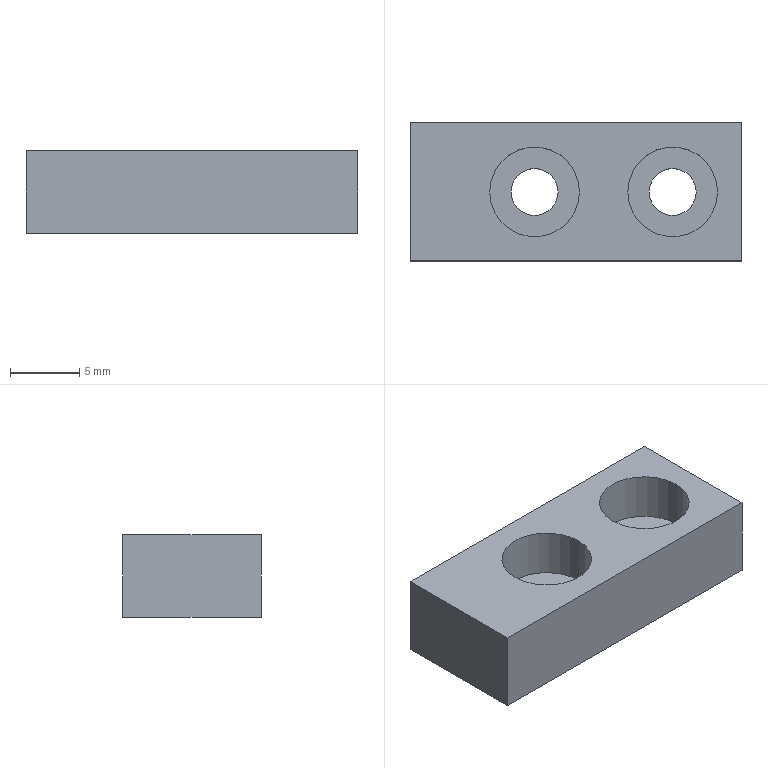Part | STEP file | 0232_211_Slide_Plate | 1 solid | 16 faces | box 24 x 10 x 6 mm | volume 1162 mm3 | cylinder 8 | plane 8 | commonest cylinder face diameters 3.4 x4 6.5 x4
STEP:
#1=CARTESIAN_POINT('',(0.,0.,0.));
#2=DIRECTION('',(0.,0.,1.));
#3=DIRECTION('',(1.,0.,0.));
#4=AXIS2_PLACEMENT_3D('',#1,#2,#3);
#5=CARTESIAN_POINT('',(-11.75,5.,2.5));
#6=VERTEX_POINT('',#5);
#7=CARTESIAN_POINT('',(-11.75,5.,6.));
#8=VERTEX_POINT('',#7);
#9=CARTESIAN_POINT('',(-11.75,5.,6.));
#10=DIRECTION('',(0.,0.,1.));
#11=VECTOR('',#10,1.);
#12=LINE('',#9,#11);
#13=CARTESIAN_POINT('',(-15.,5.,6.));
#14=DIRECTION('',(0.,0.,1.));
#15=DIRECTION('',(1.,0.,0.));
#16=AXIS2_PLACEMENT_3D('',#13,#14,#15);
#17=CYLINDRICAL_SURFACE('',#16,3.25);
#18=CARTESIAN_POINT('',(6.283,0.));
#19=DIRECTION('',(0.,1.));
#20=VECTOR('',#19,1.);
#21=LINE('',#18,#20);
#22=(GEOMETRIC_REPRESENTATION_CONTEXT(2)PARAMETRIC_REPRESENTATION_CONTEXT()REPRESENTATION_CONTEXT('',''));
#23=DEFINITIONAL_REPRESENTATION('',(#21),#22);
#24=PCURVE('',#17,#23);
#25=CARTESIAN_POINT('',(-15.,5.,6.));
#26=DIRECTION('',(0.,0.,1.));
#27=DIRECTION('',(1.,0.,0.));
#28=AXIS2_PLACEMENT_3D('',#25,#26,#27);
#29=CYLINDRICAL_SURFACE('',#28,3.25);
#30=CARTESIAN_POINT('',(0.,0.));
#31=DIRECTION('',(0.,1.));
#32=VECTOR('',#31,1.);
#33=LINE('',#30,#32);
#34=(GEOMETRIC_REPRESENTATION_CONTEXT(2)PARAMETRIC_REPRESENTATION_CONTEXT()REPRESENTATION_CONTEXT('',''));
#35=DEFINITIONAL_REPRESENTATION('',(#33),#34);
#36=PCURVE('',#29,#35);
#37=SURFACE_CURVE('',#12,(#24,#36),.PCURVE_S1.);
#38=EDGE_CURVE('',#6,#8,#37,.T.);
#39=ORIENTED_EDGE('',*,*,#38,.T.);
#40=CARTESIAN_POINT('',(-18.25,5.,6.));
#41=VERTEX_POINT('',#40);
#42=CARTESIAN_POINT('',(-15.,5.,6.));
#43=DIRECTION('',(0.,0.,1.));
#44=DIRECTION('',(1.,0.,0.));
#45=AXIS2_PLACEMENT_3D('',#42,#43,#44);
#46=CIRCLE('',#45,3.25);
#47=CARTESIAN_POINT('',(0.,0.));
#48=DIRECTION('',(1.,0.));
#49=VECTOR('',#48,1.);
#50=LINE('',#47,#49);
#51=(GEOMETRIC_REPRESENTATION_CONTEXT(2)PARAMETRIC_REPRESENTATION_CONTEXT()REPRESENTATION_CONTEXT('',''));
#52=DEFINITIONAL_REPRESENTATION('',(#50),#51);
#53=PCURVE('',#17,#52);
#54=CARTESIAN_POINT('',(-24.,0.,6.));
#55=DIRECTION('',(0.,0.,1.));
#56=DIRECTION('',(1.,0.,0.));
#57=AXIS2_PLACEMENT_3D('',#54,#55,#56);
#58=PLANE('',#57);
#59=CARTESIAN_POINT('',(9.,5.));
#60=DIRECTION('',(1.,0.));
#61=AXIS2_PLACEMENT_2D('',#59,#60);
#62=CIRCLE('',#61,3.25);
#63=(GEOMETRIC_REPRESENTATION_CONTEXT(2)PARAMETRIC_REPRESENTATION_CONTEXT()REPRESENTATION_CONTEXT('',''));
#64=DEFINITIONAL_REPRESENTATION('',(#62),#63);
#65=PCURVE('',#58,#64);
#66=SURFACE_CURVE('',#46,(#53,#65),.PCURVE_S1.);
#67=EDGE_CURVE('',#41,#8,#66,.T.);
#68=ORIENTED_EDGE('',*,*,#67,.F.);
#69=CARTESIAN_POINT('',(-18.25,5.,2.5));
#70=VERTEX_POINT('',#69);
#71=CARTESIAN_POINT('',(-18.25,5.,6.));
#72=DIRECTION('',(0.,0.,1.));
#73=VECTOR('',#72,1.);
#74=LINE('',#71,#73);
#75=CARTESIAN_POINT('',(3.142,0.));
#76=DIRECTION('',(0.,1.));
#77=VECTOR('',#76,1.);
#78=LINE('',#75,#77);
#79=(GEOMETRIC_REPRESENTATION_CONTEXT(2)PARAMETRIC_REPRESENTATION_CONTEXT()REPRESENTATION_CONTEXT('',''));
#80=DEFINITIONAL_REPRESENTATION('',(#78),#79);
#81=PCURVE('',#17,#80);
#82=CARTESIAN_POINT('',(3.142,0.));
#83=DIRECTION('',(0.,1.));
#84=VECTOR('',#83,1.);
#85=LINE('',#82,#84);
#86=(GEOMETRIC_REPRESENTATION_CONTEXT(2)PARAMETRIC_REPRESENTATION_CONTEXT()REPRESENTATION_CONTEXT('',''));
#87=DEFINITIONAL_REPRESENTATION('',(#85),#86);
#88=PCURVE('',#29,#87);
#89=SURFACE_CURVE('',#74,(#81,#88),.PCURVE_S1.);
#90=EDGE_CURVE('',#70,#41,#89,.T.);
#91=ORIENTED_EDGE('',*,*,#90,.F.);
#92=CARTESIAN_POINT('',(-15.,5.,2.5));
#93=DIRECTION('',(0.,0.,1.));
#94=DIRECTION('',(1.,0.,0.));
#95=AXIS2_PLACEMENT_3D('',#92,#93,#94);
#96=CIRCLE('',#95,3.25);
#97=CARTESIAN_POINT('',(0.,-3.5));
#98=DIRECTION('',(1.,0.));
#99=VECTOR('',#98,1.);
#100=LINE('',#97,#99);
#101=(GEOMETRIC_REPRESENTATION_CONTEXT(2)PARAMETRIC_REPRESENTATION_CONTEXT()REPRESENTATION_CONTEXT('',''));
#102=DEFINITIONAL_REPRESENTATION('',(#100),#101);
#103=PCURVE('',#17,#102);
#104=CARTESIAN_POINT('',(-13.3,5.,2.5));
#105=DIRECTION('',(0.,0.,-1.));
#106=DIRECTION('',(-1.,0.,0.));
#107=AXIS2_PLACEMENT_3D('',#104,#105,#106);
#108=PLANE('',#107);
#109=CARTESIAN_POINT('',(-1.55,0.));
#110=CARTESIAN_POINT('',(-1.55,5.629));
#111=CARTESIAN_POINT('',(3.325,2.815));
#112=CARTESIAN_POINT('',(8.2,0.));
#113=CARTESIAN_POINT('',(3.325,-2.815));
#114=CARTESIAN_POINT('',(-1.55,-5.629));
#115=CARTESIAN_POINT('',(-1.55,0.));
#116=(BOUNDED_CURVE()B_SPLINE_CURVE(2,(#109,#110,#111,#112,#113,#114,#115),.UNSPECIFIED.,.T.,.F.)B_SPLINE_CURVE_WITH_KNOTS((1,2,2,2,2,1),(-2.094,0.,2.094,4.189,6.283,8.378),.UNSPECIFIED.)CURVE()GEOMETRIC_REPRESENTATION_ITEM()RATIONAL_B_SPLINE_CURVE((1.,0.5,1.,0.5,1.,0.5,1.))REPRESENTATION_ITEM(''));
#117=(GEOMETRIC_REPRESENTATION_CONTEXT(2)PARAMETRIC_REPRESENTATION_CONTEXT()REPRESENTATION_CONTEXT('',''));
#118=DEFINITIONAL_REPRESENTATION('',(#116),#117);
#119=PCURVE('',#108,#118);
#120=SURFACE_CURVE('',#96,(#103,#119),.PCURVE_S1.);
#121=EDGE_CURVE('',#70,#6,#120,.T.);
#122=ORIENTED_EDGE('',*,*,#121,.T.);
#123=EDGE_LOOP('',(#39,#68,#91,#122));
#124=FACE_BOUND('',#123,.F.);
#125=ADVANCED_FACE('',(#124),#17,.F.);
#126=CARTESIAN_POINT('',(-13.3,5.,0.));
#127=VERTEX_POINT('',#126);
#128=CARTESIAN_POINT('',(-13.3,5.,2.5));
#129=VERTEX_POINT('',#128);
#130=CARTESIAN_POINT('',(-13.3,5.,6.));
#131=DIRECTION('',(0.,0.,1.));
#132=VECTOR('',#131,1.);
#133=LINE('',#130,#132);
#134=CARTESIAN_POINT('',(-15.,5.,6.));
#135=DIRECTION('',(0.,0.,1.));
#136=DIRECTION('',(1.,0.,0.));
#137=AXIS2_PLACEMENT_3D('',#134,#135,#136);
#138=CYLINDRICAL_SURFACE('',#137,1.7);
#139=CARTESIAN_POINT('',(6.283,0.));
#140=DIRECTION('',(0.,1.));
#141=VECTOR('',#140,1.);
#142=LINE('',#139,#141);
#143=(GEOMETRIC_REPRESENTATION_CONTEXT(2)PARAMETRIC_REPRESENTATION_CONTEXT()REPRESENTATION_CONTEXT('',''));
#144=DEFINITIONAL_REPRESENTATION('',(#142),#143);
#145=PCURVE('',#138,#144);
#146=CARTESIAN_POINT('',(-15.,5.,6.));
#147=DIRECTION('',(0.,0.,1.));
#148=DIRECTION('',(1.,0.,0.));
#149=AXIS2_PLACEMENT_3D('',#146,#147,#148);
#150=CYLINDRICAL_SURFACE('',#149,1.7);
#151=CARTESIAN_POINT('',(0.,0.));
#152=DIRECTION('',(0.,1.));
#153=VECTOR('',#152,1.);
#154=LINE('',#151,#153);
#155=(GEOMETRIC_REPRESENTATION_CONTEXT(2)PARAMETRIC_REPRESENTATION_CONTEXT()REPRESENTATION_CONTEXT('',''));
#156=DEFINITIONAL_REPRESENTATION('',(#154),#155);
#157=PCURVE('',#150,#156);
#158=SURFACE_CURVE('',#133,(#145,#157),.PCURVE_S1.);
#159=EDGE_CURVE('',#127,#129,#158,.T.);
#160=ORIENTED_EDGE('',*,*,#159,.T.);
#161=CARTESIAN_POINT('',(-16.7,5.,2.5));
#162=VERTEX_POINT('',#161);
#163=CARTESIAN_POINT('',(-15.,5.,2.5));
#164=DIRECTION('',(0.,0.,1.));
#165=DIRECTION('',(1.,0.,0.));
#166=AXIS2_PLACEMENT_3D('',#163,#164,#165);
#167=CIRCLE('',#166,1.7);
#168=CARTESIAN_POINT('',(0.,-3.5));
#169=DIRECTION('',(1.,0.));
#170=VECTOR('',#169,1.);
#171=LINE('',#168,#170);
#172=(GEOMETRIC_REPRESENTATION_CONTEXT(2)PARAMETRIC_REPRESENTATION_CONTEXT()REPRESENTATION_CONTEXT('',''));
#173=DEFINITIONAL_REPRESENTATION('',(#171),#172);
#174=PCURVE('',#138,#173);
#175=CARTESIAN_POINT('',(0.,0.));
#176=CARTESIAN_POINT('',(0.,2.944));
#177=CARTESIAN_POINT('',(2.55,1.472));
#178=CARTESIAN_POINT('',(5.1,0.));
#179=CARTESIAN_POINT('',(2.55,-1.472));
#180=CARTESIAN_POINT('',(0.,-2.944));
#181=CARTESIAN_POINT('',(0.,0.));
#182=(BOUNDED_CURVE()B_SPLINE_CURVE(2,(#175,#176,#177,#178,#179,#180,#181),.UNSPECIFIED.,.T.,.F.)B_SPLINE_CURVE_WITH_KNOTS((1,2,2,2,2,1),(-2.094,0.,2.094,4.189,6.283,8.378),.UNSPECIFIED.)CURVE()GEOMETRIC_REPRESENTATION_ITEM()RATIONAL_B_SPLINE_CURVE((1.,0.5,1.,0.5,1.,0.5,1.))REPRESENTATION_ITEM(''));
#183=(GEOMETRIC_REPRESENTATION_CONTEXT(2)PARAMETRIC_REPRESENTATION_CONTEXT()REPRESENTATION_CONTEXT('',''));
#184=DEFINITIONAL_REPRESENTATION('',(#182),#183);
#185=PCURVE('',#108,#184);
#186=SURFACE_CURVE('',#167,(#174,#185),.PCURVE_S1.);
#187=EDGE_CURVE('',#162,#129,#186,.T.);
#188=ORIENTED_EDGE('',*,*,#187,.F.);
#189=CARTESIAN_POINT('',(-16.7,5.,0.));
#190=VERTEX_POINT('',#189);
#191=CARTESIAN_POINT('',(-16.7,5.,6.));
#192=DIRECTION('',(0.,0.,1.));
#193=VECTOR('',#192,1.);
#194=LINE('',#191,#193);
#195=CARTESIAN_POINT('',(3.142,0.));
#196=DIRECTION('',(0.,1.));
#197=VECTOR('',#196,1.);
#198=LINE('',#195,#197);
#199=(GEOMETRIC_REPRESENTATION_CONTEXT(2)PARAMETRIC_REPRESENTATION_CONTEXT()REPRESENTATION_CONTEXT('',''));
#200=DEFINITIONAL_REPRESENTATION('',(#198),#199);
#201=PCURVE('',#138,#200);
#202=CARTESIAN_POINT('',(3.142,0.));
#203=DIRECTION('',(0.,1.));
#204=VECTOR('',#203,1.);
#205=LINE('',#202,#204);
#206=(GEOMETRIC_REPRESENTATION_CONTEXT(2)PARAMETRIC_REPRESENTATION_CONTEXT()REPRESENTATION_CONTEXT('',''));
#207=DEFINITIONAL_REPRESENTATION('',(#205),#206);
#208=PCURVE('',#150,#207);
#209=SURFACE_CURVE('',#194,(#201,#208),.PCURVE_S1.);
#210=EDGE_CURVE('',#190,#162,#209,.T.);
#211=ORIENTED_EDGE('',*,*,#210,.F.);
#212=CARTESIAN_POINT('',(-15.,5.,0.));
#213=DIRECTION('',(0.,0.,1.));
#214=DIRECTION('',(1.,0.,0.));
#215=AXIS2_PLACEMENT_3D('',#212,#213,#214);
#216=CIRCLE('',#215,1.7);
#217=CARTESIAN_POINT('',(0.,-6.));
#218=DIRECTION('',(1.,0.));
#219=VECTOR('',#218,1.);
#220=LINE('',#217,#219);
#221=(GEOMETRIC_REPRESENTATION_CONTEXT(2)PARAMETRIC_REPRESENTATION_CONTEXT()REPRESENTATION_CONTEXT('',''));
#222=DEFINITIONAL_REPRESENTATION('',(#220),#221);
#223=PCURVE('',#138,#222);
#224=CARTESIAN_POINT('',(-24.,0.,0.));
#225=DIRECTION('',(0.,0.,1.));
#226=DIRECTION('',(1.,0.,0.));
#227=AXIS2_PLACEMENT_3D('',#224,#225,#226);
#228=PLANE('',#227);
#229=CARTESIAN_POINT('',(9.,5.));
#230=DIRECTION('',(1.,0.));
#231=AXIS2_PLACEMENT_2D('',#229,#230);
#232=CIRCLE('',#231,1.7);
#233=(GEOMETRIC_REPRESENTATION_CONTEXT(2)PARAMETRIC_REPRESENTATION_CONTEXT()REPRESENTATION_CONTEXT('',''));
#234=DEFINITIONAL_REPRESENTATION('',(#232),#233);
#235=PCURVE('',#228,#234);
#236=SURFACE_CURVE('',#216,(#223,#235),.PCURVE_S1.);
#237=EDGE_CURVE('',#190,#127,#236,.T.);
#238=ORIENTED_EDGE('',*,*,#237,.T.);
#239=EDGE_LOOP('',(#160,#188,#211,#238));
#240=FACE_BOUND('',#239,.F.);
#241=ADVANCED_FACE('',(#240),#138,.F.);
#242=CARTESIAN_POINT('',(-1.75,5.,2.5));
#243=VERTEX_POINT('',#242);
#244=CARTESIAN_POINT('',(-1.75,5.,6.));
#245=VERTEX_POINT('',#244);
#246=CARTESIAN_POINT('',(-1.75,5.,6.));
#247=DIRECTION('',(0.,0.,1.));
#248=VECTOR('',#247,1.);
#249=LINE('',#246,#248);
#250=CARTESIAN_POINT('',(-5.,5.,6.));
#251=DIRECTION('',(0.,0.,1.));
#252=DIRECTION('',(1.,0.,0.));
#253=AXIS2_PLACEMENT_3D('',#250,#251,#252);
#254=CYLINDRICAL_SURFACE('',#253,3.25);
#255=CARTESIAN_POINT('',(6.283,0.));
#256=DIRECTION('',(0.,1.));
#257=VECTOR('',#256,1.);
#258=LINE('',#255,#257);
#259=(GEOMETRIC_REPRESENTATION_CONTEXT(2)PARAMETRIC_REPRESENTATION_CONTEXT()REPRESENTATION_CONTEXT('',''));
#260=DEFINITIONAL_REPRESENTATION('',(#258),#259);
#261=PCURVE('',#254,#260);
#262=CARTESIAN_POINT('',(-5.,5.,6.));
#263=DIRECTION('',(0.,0.,1.));
#264=DIRECTION('',(1.,0.,0.));
#265=AXIS2_PLACEMENT_3D('',#262,#263,#264);
#266=CYLINDRICAL_SURFACE('',#265,3.25);
#267=CARTESIAN_POINT('',(0.,0.));
#268=DIRECTION('',(0.,1.));
#269=VECTOR('',#268,1.);
#270=LINE('',#267,#269);
#271=(GEOMETRIC_REPRESENTATION_CONTEXT(2)PARAMETRIC_REPRESENTATION_CONTEXT()REPRESENTATION_CONTEXT('',''));
#272=DEFINITIONAL_REPRESENTATION('',(#270),#271);
#273=PCURVE('',#266,#272);
#274=SURFACE_CURVE('',#249,(#261,#273),.PCURVE_S1.);
#275=EDGE_CURVE('',#243,#245,#274,.T.);
#276=ORIENTED_EDGE('',*,*,#275,.T.);
#277=CARTESIAN_POINT('',(-8.25,5.,6.));
#278=VERTEX_POINT('',#277);
#279=CARTESIAN_POINT('',(-5.,5.,6.));
#280=DIRECTION('',(0.,0.,1.));
#281=DIRECTION('',(1.,0.,0.));
#282=AXIS2_PLACEMENT_3D('',#279,#280,#281);
#283=CIRCLE('',#282,3.25);
#284=CARTESIAN_POINT('',(0.,0.));
#285=DIRECTION('',(1.,0.));
#286=VECTOR('',#285,1.);
#287=LINE('',#284,#286);
#288=(GEOMETRIC_REPRESENTATION_CONTEXT(2)PARAMETRIC_REPRESENTATION_CONTEXT()REPRESENTATION_CONTEXT('',''));
#289=DEFINITIONAL_REPRESENTATION('',(#287),#288);
#290=PCURVE('',#254,#289);
#291=CARTESIAN_POINT('',(19.,5.));
#292=DIRECTION('',(1.,0.));
#293=AXIS2_PLACEMENT_2D('',#291,#292);
#294=CIRCLE('',#293,3.25);
#295=(GEOMETRIC_REPRESENTATION_CONTEXT(2)PARAMETRIC_REPRESENTATION_CONTEXT()REPRESENTATION_CONTEXT('',''));
#296=DEFINITIONAL_REPRESENTATION('',(#294),#295);
#297=PCURVE('',#58,#296);
#298=SURFACE_CURVE('',#283,(#290,#297),.PCURVE_S1.);
#299=EDGE_CURVE('',#278,#245,#298,.T.);
#300=ORIENTED_EDGE('',*,*,#299,.F.);
#301=CARTESIAN_POINT('',(-8.25,5.,2.5));
#302=VERTEX_POINT('',#301);
#303=CARTESIAN_POINT('',(-8.25,5.,6.));
#304=DIRECTION('',(0.,0.,1.));
#305=VECTOR('',#304,1.);
#306=LINE('',#303,#305);
#307=CARTESIAN_POINT('',(3.142,0.));
#308=DIRECTION('',(0.,1.));
#309=VECTOR('',#308,1.);
#310=LINE('',#307,#309);
#311=(GEOMETRIC_REPRESENTATION_CONTEXT(2)PARAMETRIC_REPRESENTATION_CONTEXT()REPRESENTATION_CONTEXT('',''));
#312=DEFINITIONAL_REPRESENTATION('',(#310),#311);
#313=PCURVE('',#254,#312);
#314=CARTESIAN_POINT('',(3.142,0.));
#315=DIRECTION('',(0.,1.));
#316=VECTOR('',#315,1.);
#317=LINE('',#314,#316);
#318=(GEOMETRIC_REPRESENTATION_CONTEXT(2)PARAMETRIC_REPRESENTATION_CONTEXT()REPRESENTATION_CONTEXT('',''));
#319=DEFINITIONAL_REPRESENTATION('',(#317),#318);
#320=PCURVE('',#266,#319);
#321=SURFACE_CURVE('',#306,(#313,#320),.PCURVE_S1.);
#322=EDGE_CURVE('',#302,#278,#321,.T.);
#323=ORIENTED_EDGE('',*,*,#322,.F.);
#324=CARTESIAN_POINT('',(-5.,5.,2.5));
#325=DIRECTION('',(0.,0.,1.));
#326=DIRECTION('',(1.,0.,0.));
#327=AXIS2_PLACEMENT_3D('',#324,#325,#326);
#328=CIRCLE('',#327,3.25);
#329=CARTESIAN_POINT('',(0.,-3.5));
#330=DIRECTION('',(1.,0.));
#331=VECTOR('',#330,1.);
#332=LINE('',#329,#331);
#333=(GEOMETRIC_REPRESENTATION_CONTEXT(2)PARAMETRIC_REPRESENTATION_CONTEXT()REPRESENTATION_CONTEXT('',''));
#334=DEFINITIONAL_REPRESENTATION('',(#332),#333);
#335=PCURVE('',#254,#334);
#336=CARTESIAN_POINT('',(-3.3,5.,2.5));
#337=DIRECTION('',(0.,0.,-1.));
#338=DIRECTION('',(-1.,0.,0.));
#339=AXIS2_PLACEMENT_3D('',#336,#337,#338);
#340=PLANE('',#339);
#341=CARTESIAN_POINT('',(-1.55,0.));
#342=CARTESIAN_POINT('',(-1.55,5.629));
#343=CARTESIAN_POINT('',(3.325,2.815));
#344=CARTESIAN_POINT('',(8.2,0.));
#345=CARTESIAN_POINT('',(3.325,-2.815));
#346=CARTESIAN_POINT('',(-1.55,-5.629));
#347=CARTESIAN_POINT('',(-1.55,0.));
#348=(BOUNDED_CURVE()B_SPLINE_CURVE(2,(#341,#342,#343,#344,#345,#346,#347),.UNSPECIFIED.,.T.,.F.)B_SPLINE_CURVE_WITH_KNOTS((1,2,2,2,2,1),(-2.094,0.,2.094,4.189,6.283,8.378),.UNSPECIFIED.)CURVE()GEOMETRIC_REPRESENTATION_ITEM()RATIONAL_B_SPLINE_CURVE((1.,0.5,1.,0.5,1.,0.5,1.))REPRESENTATION_ITEM(''));
#349=(GEOMETRIC_REPRESENTATION_CONTEXT(2)PARAMETRIC_REPRESENTATION_CONTEXT()REPRESENTATION_CONTEXT('',''));
#350=DEFINITIONAL_REPRESENTATION('',(#348),#349);
#351=PCURVE('',#340,#350);
#352=SURFACE_CURVE('',#328,(#335,#351),.PCURVE_S1.);
#353=EDGE_CURVE('',#302,#243,#352,.T.);
#354=ORIENTED_EDGE('',*,*,#353,.T.);
#355=EDGE_LOOP('',(#276,#300,#323,#354));
#356=FACE_BOUND('',#355,.F.);
#357=ADVANCED_FACE('',(#356),#254,.F.);
#358=CARTESIAN_POINT('',(-3.3,5.,0.));
#359=VERTEX_POINT('',#358);
#360=CARTESIAN_POINT('',(-3.3,5.,2.5));
#361=VERTEX_POINT('',#360);
#362=CARTESIAN_POINT('',(-3.3,5.,6.));
#363=DIRECTION('',(0.,0.,1.));
#364=VECTOR('',#363,1.);
#365=LINE('',#362,#364);
#366=CARTESIAN_POINT('',(-5.,5.,6.));
#367=DIRECTION('',(0.,0.,1.));
#368=DIRECTION('',(1.,0.,0.));
#369=AXIS2_PLACEMENT_3D('',#366,#367,#368);
#370=CYLINDRICAL_SURFACE('',#369,1.7);
#371=CARTESIAN_POINT('',(6.283,0.));
#372=DIRECTION('',(0.,1.));
#373=VECTOR('',#372,1.);
#374=LINE('',#371,#373);
#375=(GEOMETRIC_REPRESENTATION_CONTEXT(2)PARAMETRIC_REPRESENTATION_CONTEXT()REPRESENTATION_CONTEXT('',''));
#376=DEFINITIONAL_REPRESENTATION('',(#374),#375);
#377=PCURVE('',#370,#376);
#378=CARTESIAN_POINT('',(-5.,5.,6.));
#379=DIRECTION('',(0.,0.,1.));
#380=DIRECTION('',(1.,0.,0.));
#381=AXIS2_PLACEMENT_3D('',#378,#379,#380);
#382=CYLINDRICAL_SURFACE('',#381,1.7);
#383=CARTESIAN_POINT('',(0.,0.));
#384=DIRECTION('',(0.,1.));
#385=VECTOR('',#384,1.);
#386=LINE('',#383,#385);
#387=(GEOMETRIC_REPRESENTATION_CONTEXT(2)PARAMETRIC_REPRESENTATION_CONTEXT()REPRESENTATION_CONTEXT('',''));
#388=DEFINITIONAL_REPRESENTATION('',(#386),#387);
#389=PCURVE('',#382,#388);
#390=SURFACE_CURVE('',#365,(#377,#389),.PCURVE_S1.);
#391=EDGE_CURVE('',#359,#361,#390,.T.);
#392=ORIENTED_EDGE('',*,*,#391,.T.);
#393=CARTESIAN_POINT('',(-6.7,5.,2.5));
#394=VERTEX_POINT('',#393);
#395=CARTESIAN_POINT('',(-5.,5.,2.5));
#396=DIRECTION('',(0.,0.,1.));
#397=DIRECTION('',(1.,0.,0.));
#398=AXIS2_PLACEMENT_3D('',#395,#396,#397);
#399=CIRCLE('',#398,1.7);
#400=CARTESIAN_POINT('',(0.,-3.5));
#401=DIRECTION('',(1.,0.));
#402=VECTOR('',#401,1.);
#403=LINE('',#400,#402);
#404=(GEOMETRIC_REPRESENTATION_CONTEXT(2)PARAMETRIC_REPRESENTATION_CONTEXT()REPRESENTATION_CONTEXT('',''));
#405=DEFINITIONAL_REPRESENTATION('',(#403),#404);
#406=PCURVE('',#370,#405);
#407=CARTESIAN_POINT('',(0.,0.));
#408=CARTESIAN_POINT('',(0.,2.944));
#409=CARTESIAN_POINT('',(2.55,1.472));
#410=CARTESIAN_POINT('',(5.1,0.));
#411=CARTESIAN_POINT('',(2.55,-1.472));
#412=CARTESIAN_POINT('',(0.,-2.944));
#413=CARTESIAN_POINT('',(0.,0.));
#414=(BOUNDED_CURVE()B_SPLINE_CURVE(2,(#407,#408,#409,#410,#411,#412,#413),.UNSPECIFIED.,.T.,.F.)B_SPLINE_CURVE_WITH_KNOTS((1,2,2,2,2,1),(-2.094,0.,2.094,4.189,6.283,8.378),.UNSPECIFIED.)CURVE()GEOMETRIC_REPRESENTATION_ITEM()RATIONAL_B_SPLINE_CURVE((1.,0.5,1.,0.5,1.,0.5,1.))REPRESENTATION_ITEM(''));
#415=(GEOMETRIC_REPRESENTATION_CONTEXT(2)PARAMETRIC_REPRESENTATION_CONTEXT()REPRESENTATION_CONTEXT('',''));
#416=DEFINITIONAL_REPRESENTATION('',(#414),#415);
#417=PCURVE('',#340,#416);
#418=SURFACE_CURVE('',#399,(#406,#417),.PCURVE_S1.);
#419=EDGE_CURVE('',#394,#361,#418,.T.);
#420=ORIENTED_EDGE('',*,*,#419,.F.);
#421=CARTESIAN_POINT('',(-6.7,5.,0.));
#422=VERTEX_POINT('',#421);
#423=CARTESIAN_POINT('',(-6.7,5.,6.));
#424=DIRECTION('',(0.,0.,1.));
#425=VECTOR('',#424,1.);
#426=LINE('',#423,#425);
#427=CARTESIAN_POINT('',(3.142,0.));
#428=DIRECTION('',(0.,1.));
#429=VECTOR('',#428,1.);
#430=LINE('',#427,#429);
#431=(GEOMETRIC_REPRESENTATION_CONTEXT(2)PARAMETRIC_REPRESENTATION_CONTEXT()REPRESENTATION_CONTEXT('',''));
#432=DEFINITIONAL_REPRESENTATION('',(#430),#431);
#433=PCURVE('',#370,#432);
#434=CARTESIAN_POINT('',(3.142,0.));
#435=DIRECTION('',(0.,1.));
#436=VECTOR('',#435,1.);
#437=LINE('',#434,#436);
#438=(GEOMETRIC_REPRESENTATION_CONTEXT(2)PARAMETRIC_REPRESENTATION_CONTEXT()REPRESENTATION_CONTEXT('',''));
#439=DEFINITIONAL_REPRESENTATION('',(#437),#438);
#440=PCURVE('',#382,#439);
#441=SURFACE_CURVE('',#426,(#433,#440),.PCURVE_S1.);
#442=EDGE_CURVE('',#422,#394,#441,.T.);
#443=ORIENTED_EDGE('',*,*,#442,.F.);
#444=CARTESIAN_POINT('',(-5.,5.,0.));
#445=DIRECTION('',(0.,0.,1.));
#446=DIRECTION('',(1.,0.,0.));
#447=AXIS2_PLACEMENT_3D('',#444,#445,#446);
#448=CIRCLE('',#447,1.7);
#449=CARTESIAN_POINT('',(0.,-6.));
#450=DIRECTION('',(1.,0.));
#451=VECTOR('',#450,1.);
#452=LINE('',#449,#451);
#453=(GEOMETRIC_REPRESENTATION_CONTEXT(2)PARAMETRIC_REPRESENTATION_CONTEXT()REPRESENTATION_CONTEXT('',''));
#454=DEFINITIONAL_REPRESENTATION('',(#452),#453);
#455=PCURVE('',#370,#454);
#456=CARTESIAN_POINT('',(19.,5.));
#457=DIRECTION('',(1.,0.));
#458=AXIS2_PLACEMENT_2D('',#456,#457);
#459=CIRCLE('',#458,1.7);
#460=(GEOMETRIC_REPRESENTATION_CONTEXT(2)PARAMETRIC_REPRESENTATION_CONTEXT()REPRESENTATION_CONTEXT('',''));
#461=DEFINITIONAL_REPRESENTATION('',(#459),#460);
#462=PCURVE('',#228,#461);
#463=SURFACE_CURVE('',#448,(#455,#462),.PCURVE_S1.);
#464=EDGE_CURVE('',#422,#359,#463,.T.);
#465=ORIENTED_EDGE('',*,*,#464,.T.);
#466=EDGE_LOOP('',(#392,#420,#443,#465));
#467=FACE_BOUND('',#466,.F.);
#468=ADVANCED_FACE('',(#467),#370,.F.);
#469=CARTESIAN_POINT('',(-24.,10.,0.));
#470=VERTEX_POINT('',#469);
#471=CARTESIAN_POINT('',(-24.,0.,0.));
#472=VERTEX_POINT('',#471);
#473=CARTESIAN_POINT('',(-24.,10.,0.));
#474=DIRECTION('',(0.,-1.,0.));
#475=VECTOR('',#474,1.);
#476=LINE('',#473,#475);
#477=CARTESIAN_POINT('',(-24.,10.,6.));
#478=DIRECTION('',(1.,0.,0.));
#479=DIRECTION('',(0.,0.,-1.));
#480=AXIS2_PLACEMENT_3D('',#477,#478,#479);
#481=PLANE('',#480);
#482=CARTESIAN_POINT('',(6.,0.));
#483=DIRECTION('',(0.,-1.));
#484=VECTOR('',#483,1.);
#485=LINE('',#482,#484);
#486=(GEOMETRIC_REPRESENTATION_CONTEXT(2)PARAMETRIC_REPRESENTATION_CONTEXT()REPRESENTATION_CONTEXT('',''));
#487=DEFINITIONAL_REPRESENTATION('',(#485),#486);
#488=PCURVE('',#481,#487);
#489=CARTESIAN_POINT('',(0.,10.));
#490=DIRECTION('',(0.,-1.));
#491=VECTOR('',#490,1.);
#492=LINE('',#489,#491);
#493=(GEOMETRIC_REPRESENTATION_CONTEXT(2)PARAMETRIC_REPRESENTATION_CONTEXT()REPRESENTATION_CONTEXT('',''));
#494=DEFINITIONAL_REPRESENTATION('',(#492),#493);
#495=PCURVE('',#228,#494);
#496=SURFACE_CURVE('',#476,(#488,#495),.PCURVE_S1.);
#497=EDGE_CURVE('',#470,#472,#496,.T.);
#498=ORIENTED_EDGE('',*,*,#497,.T.);
#499=CARTESIAN_POINT('',(-24.,0.,6.));
#500=VERTEX_POINT('',#499);
#501=CARTESIAN_POINT('',(-24.,0.,6.));
#502=DIRECTION('',(0.,0.,-1.));
#503=VECTOR('',#502,1.);
#504=LINE('',#501,#503);
#505=CARTESIAN_POINT('',(0.,-10.));
#506=DIRECTION('',(1.,0.));
#507=VECTOR('',#506,1.);
#508=LINE('',#505,#507);
#509=(GEOMETRIC_REPRESENTATION_CONTEXT(2)PARAMETRIC_REPRESENTATION_CONTEXT()REPRESENTATION_CONTEXT('',''));
#510=DEFINITIONAL_REPRESENTATION('',(#508),#509);
#511=PCURVE('',#481,#510);
#512=CARTESIAN_POINT('',(-24.,0.,6.));
#513=DIRECTION('',(0.,1.,0.));
#514=DIRECTION('',(0.,0.,1.));
#515=AXIS2_PLACEMENT_3D('',#512,#513,#514);
#516=PLANE('',#515);
#517=CARTESIAN_POINT('',(0.,0.));
#518=DIRECTION('',(-1.,0.));
#519=VECTOR('',#518,1.);
#520=LINE('',#517,#519);
#521=(GEOMETRIC_REPRESENTATION_CONTEXT(2)PARAMETRIC_REPRESENTATION_CONTEXT()REPRESENTATION_CONTEXT('',''));
#522=DEFINITIONAL_REPRESENTATION('',(#520),#521);
#523=PCURVE('',#516,#522);
#524=SURFACE_CURVE('',#504,(#511,#523),.PCURVE_S1.);
#525=EDGE_CURVE('',#500,#472,#524,.T.);
#526=ORIENTED_EDGE('',*,*,#525,.F.);
#527=CARTESIAN_POINT('',(-24.,10.,6.));
#528=VERTEX_POINT('',#527);
#529=CARTESIAN_POINT('',(-24.,10.,6.));
#530=DIRECTION('',(0.,-1.,0.));
#531=VECTOR('',#530,1.);
#532=LINE('',#529,#531);
#533=CARTESIAN_POINT('',(0.,0.));
#534=DIRECTION('',(0.,-1.));
#535=VECTOR('',#534,1.);
#536=LINE('',#533,#535);
#537=(GEOMETRIC_REPRESENTATION_CONTEXT(2)PARAMETRIC_REPRESENTATION_CONTEXT()REPRESENTATION_CONTEXT('',''));
#538=DEFINITIONAL_REPRESENTATION('',(#536),#537);
#539=PCURVE('',#481,#538);
#540=CARTESIAN_POINT('',(0.,10.));
#541=DIRECTION('',(0.,-1.));
#542=VECTOR('',#541,1.);
#543=LINE('',#540,#542);
#544=(GEOMETRIC_REPRESENTATION_CONTEXT(2)PARAMETRIC_REPRESENTATION_CONTEXT()REPRESENTATION_CONTEXT('',''));
#545=DEFINITIONAL_REPRESENTATION('',(#543),#544);
#546=PCURVE('',#58,#545);
#547=SURFACE_CURVE('',#532,(#539,#546),.PCURVE_S1.);
#548=EDGE_CURVE('',#528,#500,#547,.T.);
#549=ORIENTED_EDGE('',*,*,#548,.F.);
#550=CARTESIAN_POINT('',(-24.,10.,6.));
#551=DIRECTION('',(0.,0.,-1.));
#552=VECTOR('',#551,1.);
#553=LINE('',#550,#552);
#554=CARTESIAN_POINT('',(0.,0.));
#555=DIRECTION('',(1.,0.));
#556=VECTOR('',#555,1.);
#557=LINE('',#554,#556);
#558=(GEOMETRIC_REPRESENTATION_CONTEXT(2)PARAMETRIC_REPRESENTATION_CONTEXT()REPRESENTATION_CONTEXT('',''));
#559=DEFINITIONAL_REPRESENTATION('',(#557),#558);
#560=PCURVE('',#481,#559);
#561=CARTESIAN_POINT('',(-24.,10.,6.));
#562=DIRECTION('',(0.,-1.,0.));
#563=DIRECTION('',(0.,0.,-1.));
#564=AXIS2_PLACEMENT_3D('',#561,#562,#563);
#565=PLANE('',#564);
#566=CARTESIAN_POINT('',(0.,0.));
#567=DIRECTION('',(1.,0.));
#568=VECTOR('',#567,1.);
#569=LINE('',#566,#568);
#570=(GEOMETRIC_REPRESENTATION_CONTEXT(2)PARAMETRIC_REPRESENTATION_CONTEXT()REPRESENTATION_CONTEXT('',''));
#571=DEFINITIONAL_REPRESENTATION('',(#569),#570);
#572=PCURVE('',#565,#571);
#573=SURFACE_CURVE('',#553,(#560,#572),.PCURVE_S1.);
#574=EDGE_CURVE('',#528,#470,#573,.T.);
#575=ORIENTED_EDGE('',*,*,#574,.T.);
#576=EDGE_LOOP('',(#498,#526,#549,#575));
#577=FACE_BOUND('',#576,.T.);
#578=ADVANCED_FACE('',(#577),#481,.F.);
#579=CARTESIAN_POINT('',(0.,0.,0.));
#580=VERTEX_POINT('',#579);
#581=CARTESIAN_POINT('',(-24.,0.,0.));
#582=DIRECTION('',(1.,0.,0.));
#583=VECTOR('',#582,1.);
#584=LINE('',#581,#583);
#585=CARTESIAN_POINT('',(-6.,0.));
#586=DIRECTION('',(0.,1.));
#587=VECTOR('',#586,1.);
#588=LINE('',#585,#587);
#589=(GEOMETRIC_REPRESENTATION_CONTEXT(2)PARAMETRIC_REPRESENTATION_CONTEXT()REPRESENTATION_CONTEXT('',''));
#590=DEFINITIONAL_REPRESENTATION('',(#588),#589);
#591=PCURVE('',#516,#590);
#592=CARTESIAN_POINT('',(0.,0.));
#593=DIRECTION('',(1.,0.));
#594=VECTOR('',#593,1.);
#595=LINE('',#592,#594);
#596=(GEOMETRIC_REPRESENTATION_CONTEXT(2)PARAMETRIC_REPRESENTATION_CONTEXT()REPRESENTATION_CONTEXT('',''));
#597=DEFINITIONAL_REPRESENTATION('',(#595),#596);
#598=PCURVE('',#228,#597);
#599=SURFACE_CURVE('',#584,(#591,#598),.PCURVE_S1.);
#600=EDGE_CURVE('',#472,#580,#599,.T.);
#601=ORIENTED_EDGE('',*,*,#600,.T.);
#602=CARTESIAN_POINT('',(0.,0.,6.));
#603=VERTEX_POINT('',#602);
#604=CARTESIAN_POINT('',(0.,0.,6.));
#605=DIRECTION('',(0.,0.,-1.));
#606=VECTOR('',#605,1.);
#607=LINE('',#604,#606);
#608=CARTESIAN_POINT('',(0.,24.));
#609=DIRECTION('',(-1.,0.));
#610=VECTOR('',#609,1.);
#611=LINE('',#608,#610);
#612=(GEOMETRIC_REPRESENTATION_CONTEXT(2)PARAMETRIC_REPRESENTATION_CONTEXT()REPRESENTATION_CONTEXT('',''));
#613=DEFINITIONAL_REPRESENTATION('',(#611),#612);
#614=PCURVE('',#516,#613);
#615=CARTESIAN_POINT('',(0.,10.,6.));
#616=DIRECTION('',(-1.,0.,0.));
#617=DIRECTION('',(0.,-1.,0.));
#618=AXIS2_PLACEMENT_3D('',#615,#616,#617);
#619=PLANE('',#618);
#620=CARTESIAN_POINT('',(10.,0.));
#621=DIRECTION('',(0.,-1.));
#622=VECTOR('',#621,1.);
#623=LINE('',#620,#622);
#624=(GEOMETRIC_REPRESENTATION_CONTEXT(2)PARAMETRIC_REPRESENTATION_CONTEXT()REPRESENTATION_CONTEXT('',''));
#625=DEFINITIONAL_REPRESENTATION('',(#623),#624);
#626=PCURVE('',#619,#625);
#627=SURFACE_CURVE('',#607,(#614,#626),.PCURVE_S1.);
#628=EDGE_CURVE('',#603,#580,#627,.T.);
#629=ORIENTED_EDGE('',*,*,#628,.F.);
#630=CARTESIAN_POINT('',(-24.,0.,6.));
#631=DIRECTION('',(1.,0.,0.));
#632=VECTOR('',#631,1.);
#633=LINE('',#630,#632);
#634=CARTESIAN_POINT('',(0.,0.));
#635=DIRECTION('',(0.,1.));
#636=VECTOR('',#635,1.);
#637=LINE('',#634,#636);
#638=(GEOMETRIC_REPRESENTATION_CONTEXT(2)PARAMETRIC_REPRESENTATION_CONTEXT()REPRESENTATION_CONTEXT('',''));
#639=DEFINITIONAL_REPRESENTATION('',(#637),#638);
#640=PCURVE('',#516,#639);
#641=CARTESIAN_POINT('',(0.,0.));
#642=DIRECTION('',(1.,0.));
#643=VECTOR('',#642,1.);
#644=LINE('',#641,#643);
#645=(GEOMETRIC_REPRESENTATION_CONTEXT(2)PARAMETRIC_REPRESENTATION_CONTEXT()REPRESENTATION_CONTEXT('',''));
#646=DEFINITIONAL_REPRESENTATION('',(#644),#645);
#647=PCURVE('',#58,#646);
#648=SURFACE_CURVE('',#633,(#640,#647),.PCURVE_S1.);
#649=EDGE_CURVE('',#500,#603,#648,.T.);
#650=ORIENTED_EDGE('',*,*,#649,.F.);
#651=ORIENTED_EDGE('',*,*,#525,.T.);
#652=EDGE_LOOP('',(#601,#629,#650,#651));
#653=FACE_BOUND('',#652,.T.);
#654=ADVANCED_FACE('',(#653),#516,.F.);
#655=CARTESIAN_POINT('',(0.,10.,0.));
#656=VERTEX_POINT('',#655);
#657=CARTESIAN_POINT('',(0.,10.,0.));
#658=DIRECTION('',(0.,1.,0.));
#659=VECTOR('',#658,1.);
#660=LINE('',#657,#659);
#661=CARTESIAN_POINT('',(0.,-6.));
#662=DIRECTION('',(-1.,0.));
#663=VECTOR('',#662,1.);
#664=LINE('',#661,#663);
#665=(GEOMETRIC_REPRESENTATION_CONTEXT(2)PARAMETRIC_REPRESENTATION_CONTEXT()REPRESENTATION_CONTEXT('',''));
#666=DEFINITIONAL_REPRESENTATION('',(#664),#665);
#667=PCURVE('',#619,#666);
#668=CARTESIAN_POINT('',(24.,10.));
#669=DIRECTION('',(0.,1.));
#670=VECTOR('',#669,1.);
#671=LINE('',#668,#670);
#672=(GEOMETRIC_REPRESENTATION_CONTEXT(2)PARAMETRIC_REPRESENTATION_CONTEXT()REPRESENTATION_CONTEXT('',''));
#673=DEFINITIONAL_REPRESENTATION('',(#671),#672);
#674=PCURVE('',#228,#673);
#675=SURFACE_CURVE('',#660,(#667,#674),.PCURVE_S1.);
#676=EDGE_CURVE('',#580,#656,#675,.T.);
#677=ORIENTED_EDGE('',*,*,#676,.T.);
#678=CARTESIAN_POINT('',(0.,10.,6.));
#679=VERTEX_POINT('',#678);
#680=CARTESIAN_POINT('',(0.,10.,6.));
#681=DIRECTION('',(0.,0.,-1.));
#682=VECTOR('',#681,1.);
#683=LINE('',#680,#682);
#684=CARTESIAN_POINT('',(0.,0.));
#685=DIRECTION('',(0.,-1.));
#686=VECTOR('',#685,1.);
#687=LINE('',#684,#686);
#688=(GEOMETRIC_REPRESENTATION_CONTEXT(2)PARAMETRIC_REPRESENTATION_CONTEXT()REPRESENTATION_CONTEXT('',''));
#689=DEFINITIONAL_REPRESENTATION('',(#687),#688);
#690=PCURVE('',#619,#689);
#691=CARTESIAN_POINT('',(0.,24.));
#692=DIRECTION('',(1.,0.));
#693=VECTOR('',#692,1.);
#694=LINE('',#691,#693);
#695=(GEOMETRIC_REPRESENTATION_CONTEXT(2)PARAMETRIC_REPRESENTATION_CONTEXT()REPRESENTATION_CONTEXT('',''));
#696=DEFINITIONAL_REPRESENTATION('',(#694),#695);
#697=PCURVE('',#565,#696);
#698=SURFACE_CURVE('',#683,(#690,#697),.PCURVE_S1.);
#699=EDGE_CURVE('',#679,#656,#698,.T.);
#700=ORIENTED_EDGE('',*,*,#699,.F.);
#701=CARTESIAN_POINT('',(0.,10.,6.));
#702=DIRECTION('',(0.,1.,0.));
#703=VECTOR('',#702,1.);
#704=LINE('',#701,#703);
#705=CARTESIAN_POINT('',(0.,0.));
#706=DIRECTION('',(-1.,0.));
#707=VECTOR('',#706,1.);
#708=LINE('',#705,#707);
#709=(GEOMETRIC_REPRESENTATION_CONTEXT(2)PARAMETRIC_REPRESENTATION_CONTEXT()REPRESENTATION_CONTEXT('',''));
#710=DEFINITIONAL_REPRESENTATION('',(#708),#709);
#711=PCURVE('',#619,#710);
#712=CARTESIAN_POINT('',(24.,10.));
#713=DIRECTION('',(0.,1.));
#714=VECTOR('',#713,1.);
#715=LINE('',#712,#714);
#716=(GEOMETRIC_REPRESENTATION_CONTEXT(2)PARAMETRIC_REPRESENTATION_CONTEXT()REPRESENTATION_CONTEXT('',''));
#717=DEFINITIONAL_REPRESENTATION('',(#715),#716);
#718=PCURVE('',#58,#717);
#719=SURFACE_CURVE('',#704,(#711,#718),.PCURVE_S1.);
#720=EDGE_CURVE('',#603,#679,#719,.T.);
#721=ORIENTED_EDGE('',*,*,#720,.F.);
#722=ORIENTED_EDGE('',*,*,#628,.T.);
#723=EDGE_LOOP('',(#677,#700,#721,#722));
#724=FACE_BOUND('',#723,.T.);
#725=ADVANCED_FACE('',(#724),#619,.F.);
#726=CARTESIAN_POINT('',(-24.,10.,0.));
#727=DIRECTION('',(-1.,0.,0.));
#728=VECTOR('',#727,1.);
#729=LINE('',#726,#728);
#730=CARTESIAN_POINT('',(6.,0.));
#731=DIRECTION('',(0.,-1.));
#732=VECTOR('',#731,1.);
#733=LINE('',#730,#732);
#734=(GEOMETRIC_REPRESENTATION_CONTEXT(2)PARAMETRIC_REPRESENTATION_CONTEXT()REPRESENTATION_CONTEXT('',''));
#735=DEFINITIONAL_REPRESENTATION('',(#733),#734);
#736=PCURVE('',#565,#735);
#737=CARTESIAN_POINT('',(0.,10.));
#738=DIRECTION('',(-1.,0.));
#739=VECTOR('',#738,1.);
#740=LINE('',#737,#739);
#741=(GEOMETRIC_REPRESENTATION_CONTEXT(2)PARAMETRIC_REPRESENTATION_CONTEXT()REPRESENTATION_CONTEXT('',''));
#742=DEFINITIONAL_REPRESENTATION('',(#740),#741);
#743=PCURVE('',#228,#742);
#744=SURFACE_CURVE('',#729,(#736,#743),.PCURVE_S1.);
#745=EDGE_CURVE('',#656,#470,#744,.T.);
#746=ORIENTED_EDGE('',*,*,#745,.T.);
#747=ORIENTED_EDGE('',*,*,#574,.F.);
#748=CARTESIAN_POINT('',(-24.,10.,6.));
#749=DIRECTION('',(-1.,0.,0.));
#750=VECTOR('',#749,1.);
#751=LINE('',#748,#750);
#752=CARTESIAN_POINT('',(0.,0.));
#753=DIRECTION('',(0.,-1.));
#754=VECTOR('',#753,1.);
#755=LINE('',#752,#754);
#756=(GEOMETRIC_REPRESENTATION_CONTEXT(2)PARAMETRIC_REPRESENTATION_CONTEXT()REPRESENTATION_CONTEXT('',''));
#757=DEFINITIONAL_REPRESENTATION('',(#755),#756);
#758=PCURVE('',#565,#757);
#759=CARTESIAN_POINT('',(0.,10.));
#760=DIRECTION('',(-1.,0.));
#761=VECTOR('',#760,1.);
#762=LINE('',#759,#761);
#763=(GEOMETRIC_REPRESENTATION_CONTEXT(2)PARAMETRIC_REPRESENTATION_CONTEXT()REPRESENTATION_CONTEXT('',''));
#764=DEFINITIONAL_REPRESENTATION('',(#762),#763);
#765=PCURVE('',#58,#764);
#766=SURFACE_CURVE('',#751,(#758,#765),.PCURVE_S1.);
#767=EDGE_CURVE('',#679,#528,#766,.T.);
#768=ORIENTED_EDGE('',*,*,#767,.F.);
#769=ORIENTED_EDGE('',*,*,#699,.T.);
#770=EDGE_LOOP('',(#746,#747,#768,#769));
#771=FACE_BOUND('',#770,.T.);
#772=ADVANCED_FACE('',(#771),#565,.F.);
#773=CARTESIAN_POINT('',(-15.,5.,6.));
#774=DIRECTION('',(0.,0.,1.));
#775=DIRECTION('',(1.,0.,0.));
#776=AXIS2_PLACEMENT_3D('',#773,#774,#775);
#777=CIRCLE('',#776,3.25);
#778=CARTESIAN_POINT('',(9.,5.));
#779=DIRECTION('',(1.,0.));
#780=AXIS2_PLACEMENT_2D('',#778,#779);
#781=CIRCLE('',#780,3.25);
#782=(GEOMETRIC_REPRESENTATION_CONTEXT(2)PARAMETRIC_REPRESENTATION_CONTEXT()REPRESENTATION_CONTEXT('',''));
#783=DEFINITIONAL_REPRESENTATION('',(#781),#782);
#784=PCURVE('',#58,#783);
#785=CARTESIAN_POINT('',(0.,0.));
#786=DIRECTION('',(1.,0.));
#787=VECTOR('',#786,1.);
#788=LINE('',#785,#787);
#789=(GEOMETRIC_REPRESENTATION_CONTEXT(2)PARAMETRIC_REPRESENTATION_CONTEXT()REPRESENTATION_CONTEXT('',''));
#790=DEFINITIONAL_REPRESENTATION('',(#788),#789);
#791=PCURVE('',#29,#790);
#792=SURFACE_CURVE('',#777,(#784,#791),.PCURVE_S1.);
#793=EDGE_CURVE('',#8,#41,#792,.T.);
#794=ORIENTED_EDGE('',*,*,#793,.F.);
#795=ORIENTED_EDGE('',*,*,#67,.F.);
#796=EDGE_LOOP('',(#794,#795));
#797=FACE_BOUND('',#796,.T.);
#798=CARTESIAN_POINT('',(-5.,5.,6.));
#799=DIRECTION('',(0.,0.,1.));
#800=DIRECTION('',(1.,0.,0.));
#801=AXIS2_PLACEMENT_3D('',#798,#799,#800);
#802=CIRCLE('',#801,3.25);
#803=CARTESIAN_POINT('',(19.,5.));
#804=DIRECTION('',(1.,0.));
#805=AXIS2_PLACEMENT_2D('',#803,#804);
#806=CIRCLE('',#805,3.25);
#807=(GEOMETRIC_REPRESENTATION_CONTEXT(2)PARAMETRIC_REPRESENTATION_CONTEXT()REPRESENTATION_CONTEXT('',''));
#808=DEFINITIONAL_REPRESENTATION('',(#806),#807);
#809=PCURVE('',#58,#808);
#810=CARTESIAN_POINT('',(0.,0.));
#811=DIRECTION('',(1.,0.));
#812=VECTOR('',#811,1.);
#813=LINE('',#810,#812);
#814=(GEOMETRIC_REPRESENTATION_CONTEXT(2)PARAMETRIC_REPRESENTATION_CONTEXT()REPRESENTATION_CONTEXT('',''));
#815=DEFINITIONAL_REPRESENTATION('',(#813),#814);
#816=PCURVE('',#266,#815);
#817=SURFACE_CURVE('',#802,(#809,#816),.PCURVE_S1.);
#818=EDGE_CURVE('',#245,#278,#817,.T.);
#819=ORIENTED_EDGE('',*,*,#818,.F.);
#820=ORIENTED_EDGE('',*,*,#299,.F.);
#821=EDGE_LOOP('',(#819,#820));
#822=FACE_BOUND('',#821,.T.);
#823=ORIENTED_EDGE('',*,*,#548,.T.);
#824=ORIENTED_EDGE('',*,*,#649,.T.);
#825=ORIENTED_EDGE('',*,*,#720,.T.);
#826=ORIENTED_EDGE('',*,*,#767,.T.);
#827=EDGE_LOOP('',(#823,#824,#825,#826));
#828=FACE_BOUND('',#827,.T.);
#829=ADVANCED_FACE('',(#797,#822,#828),#58,.T.);
#830=CARTESIAN_POINT('',(-15.,5.,0.));
#831=DIRECTION('',(0.,0.,1.));
#832=DIRECTION('',(1.,0.,0.));
#833=AXIS2_PLACEMENT_3D('',#830,#831,#832);
#834=CIRCLE('',#833,1.7);
#835=CARTESIAN_POINT('',(9.,5.));
#836=DIRECTION('',(1.,0.));
#837=AXIS2_PLACEMENT_2D('',#835,#836);
#838=CIRCLE('',#837,1.7);
#839=(GEOMETRIC_REPRESENTATION_CONTEXT(2)PARAMETRIC_REPRESENTATION_CONTEXT()REPRESENTATION_CONTEXT('',''));
#840=DEFINITIONAL_REPRESENTATION('',(#838),#839);
#841=PCURVE('',#228,#840);
#842=CARTESIAN_POINT('',(0.,-6.));
#843=DIRECTION('',(1.,0.));
#844=VECTOR('',#843,1.);
#845=LINE('',#842,#844);
#846=(GEOMETRIC_REPRESENTATION_CONTEXT(2)PARAMETRIC_REPRESENTATION_CONTEXT()REPRESENTATION_CONTEXT('',''));
#847=DEFINITIONAL_REPRESENTATION('',(#845),#846);
#848=PCURVE('',#150,#847);
#849=SURFACE_CURVE('',#834,(#841,#848),.PCURVE_S1.);
#850=EDGE_CURVE('',#127,#190,#849,.T.);
#851=ORIENTED_EDGE('',*,*,#850,.T.);
#852=ORIENTED_EDGE('',*,*,#237,.T.);
#853=EDGE_LOOP('',(#851,#852));
#854=FACE_BOUND('',#853,.T.);
#855=CARTESIAN_POINT('',(-5.,5.,0.));
#856=DIRECTION('',(0.,0.,1.));
#857=DIRECTION('',(1.,0.,0.));
#858=AXIS2_PLACEMENT_3D('',#855,#856,#857);
#859=CIRCLE('',#858,1.7);
#860=CARTESIAN_POINT('',(19.,5.));
#861=DIRECTION('',(1.,0.));
#862=AXIS2_PLACEMENT_2D('',#860,#861);
#863=CIRCLE('',#862,1.7);
#864=(GEOMETRIC_REPRESENTATION_CONTEXT(2)PARAMETRIC_REPRESENTATION_CONTEXT()REPRESENTATION_CONTEXT('',''));
#865=DEFINITIONAL_REPRESENTATION('',(#863),#864);
#866=PCURVE('',#228,#865);
#867=CARTESIAN_POINT('',(0.,-6.));
#868=DIRECTION('',(1.,0.));
#869=VECTOR('',#868,1.);
#870=LINE('',#867,#869);
#871=(GEOMETRIC_REPRESENTATION_CONTEXT(2)PARAMETRIC_REPRESENTATION_CONTEXT()REPRESENTATION_CONTEXT('',''));
#872=DEFINITIONAL_REPRESENTATION('',(#870),#871);
#873=PCURVE('',#382,#872);
#874=SURFACE_CURVE('',#859,(#866,#873),.PCURVE_S1.);
#875=EDGE_CURVE('',#359,#422,#874,.T.);
#876=ORIENTED_EDGE('',*,*,#875,.T.);
#877=ORIENTED_EDGE('',*,*,#464,.T.);
#878=EDGE_LOOP('',(#876,#877));
#879=FACE_BOUND('',#878,.T.);
#880=ORIENTED_EDGE('',*,*,#497,.F.);
#881=ORIENTED_EDGE('',*,*,#745,.F.);
#882=ORIENTED_EDGE('',*,*,#676,.F.);
#883=ORIENTED_EDGE('',*,*,#600,.F.);
#884=EDGE_LOOP('',(#880,#881,#882,#883));
#885=FACE_BOUND('',#884,.T.);
#886=ADVANCED_FACE('',(#854,#879,#885),#228,.F.);
#887=CARTESIAN_POINT('',(-5.,5.,2.5));
#888=DIRECTION('',(0.,0.,1.));
#889=DIRECTION('',(1.,0.,0.));
#890=AXIS2_PLACEMENT_3D('',#887,#888,#889);
#891=CIRCLE('',#890,1.7);
#892=CARTESIAN_POINT('',(0.,-3.5));
#893=DIRECTION('',(1.,0.));
#894=VECTOR('',#893,1.);
#895=LINE('',#892,#894);
#896=(GEOMETRIC_REPRESENTATION_CONTEXT(2)PARAMETRIC_REPRESENTATION_CONTEXT()REPRESENTATION_CONTEXT('',''));
#897=DEFINITIONAL_REPRESENTATION('',(#895),#896);
#898=PCURVE('',#382,#897);
#899=CARTESIAN_POINT('',(0.,0.));
#900=CARTESIAN_POINT('',(0.,2.944));
#901=CARTESIAN_POINT('',(2.55,1.472));
#902=CARTESIAN_POINT('',(5.1,0.));
#903=CARTESIAN_POINT('',(2.55,-1.472));
#904=CARTESIAN_POINT('',(0.,-2.944));
#905=CARTESIAN_POINT('',(0.,0.));
#906=(BOUNDED_CURVE()B_SPLINE_CURVE(2,(#899,#900,#901,#902,#903,#904,#905),.UNSPECIFIED.,.T.,.F.)B_SPLINE_CURVE_WITH_KNOTS((1,2,2,2,2,1),(-2.094,0.,2.094,4.189,6.283,8.378),.UNSPECIFIED.)CURVE()GEOMETRIC_REPRESENTATION_ITEM()RATIONAL_B_SPLINE_CURVE((1.,0.5,1.,0.5,1.,0.5,1.))REPRESENTATION_ITEM(''));
#907=(GEOMETRIC_REPRESENTATION_CONTEXT(2)PARAMETRIC_REPRESENTATION_CONTEXT()REPRESENTATION_CONTEXT('',''));
#908=DEFINITIONAL_REPRESENTATION('',(#906),#907);
#909=PCURVE('',#340,#908);
#910=SURFACE_CURVE('',#891,(#898,#909),.PCURVE_S1.);
#911=EDGE_CURVE('',#361,#394,#910,.T.);
#912=ORIENTED_EDGE('',*,*,#911,.F.);
#913=ORIENTED_EDGE('',*,*,#391,.F.);
#914=ORIENTED_EDGE('',*,*,#875,.T.);
#915=ORIENTED_EDGE('',*,*,#442,.T.);
#916=EDGE_LOOP('',(#912,#913,#914,#915));
#917=FACE_BOUND('',#916,.F.);
#918=ADVANCED_FACE('',(#917),#382,.F.);
#919=ORIENTED_EDGE('',*,*,#911,.F.);
#920=ORIENTED_EDGE('',*,*,#419,.F.);
#921=EDGE_LOOP('',(#919,#920));
#922=FACE_BOUND('',#921,.T.);
#923=CARTESIAN_POINT('',(-5.,5.,2.5));
#924=DIRECTION('',(0.,0.,1.));
#925=DIRECTION('',(1.,0.,0.));
#926=AXIS2_PLACEMENT_3D('',#923,#924,#925);
#927=CIRCLE('',#926,3.25);
#928=CARTESIAN_POINT('',(-1.55,0.));
#929=CARTESIAN_POINT('',(-1.55,5.629));
#930=CARTESIAN_POINT('',(3.325,2.815));
#931=CARTESIAN_POINT('',(8.2,0.));
#932=CARTESIAN_POINT('',(3.325,-2.815));
#933=CARTESIAN_POINT('',(-1.55,-5.629));
#934=CARTESIAN_POINT('',(-1.55,0.));
#935=(BOUNDED_CURVE()B_SPLINE_CURVE(2,(#928,#929,#930,#931,#932,#933,#934),.UNSPECIFIED.,.T.,.F.)B_SPLINE_CURVE_WITH_KNOTS((1,2,2,2,2,1),(-2.094,0.,2.094,4.189,6.283,8.378),.UNSPECIFIED.)CURVE()GEOMETRIC_REPRESENTATION_ITEM()RATIONAL_B_SPLINE_CURVE((1.,0.5,1.,0.5,1.,0.5,1.))REPRESENTATION_ITEM(''));
#936=(GEOMETRIC_REPRESENTATION_CONTEXT(2)PARAMETRIC_REPRESENTATION_CONTEXT()REPRESENTATION_CONTEXT('',''));
#937=DEFINITIONAL_REPRESENTATION('',(#935),#936);
#938=PCURVE('',#340,#937);
#939=CARTESIAN_POINT('',(0.,-3.5));
#940=DIRECTION('',(1.,0.));
#941=VECTOR('',#940,1.);
#942=LINE('',#939,#941);
#943=(GEOMETRIC_REPRESENTATION_CONTEXT(2)PARAMETRIC_REPRESENTATION_CONTEXT()REPRESENTATION_CONTEXT('',''));
#944=DEFINITIONAL_REPRESENTATION('',(#942),#943);
#945=PCURVE('',#266,#944);
#946=SURFACE_CURVE('',#927,(#938,#945),.PCURVE_S1.);
#947=EDGE_CURVE('',#243,#302,#946,.T.);
#948=ORIENTED_EDGE('',*,*,#947,.T.);
#949=ORIENTED_EDGE('',*,*,#353,.T.);
#950=EDGE_LOOP('',(#948,#949));
#951=FACE_BOUND('',#950,.T.);
#952=ADVANCED_FACE('',(#922,#951),#340,.F.);
#953=ORIENTED_EDGE('',*,*,#818,.F.);
#954=ORIENTED_EDGE('',*,*,#275,.F.);
#955=ORIENTED_EDGE('',*,*,#947,.T.);
#956=ORIENTED_EDGE('',*,*,#322,.T.);
#957=EDGE_LOOP('',(#953,#954,#955,#956));
#958=FACE_BOUND('',#957,.F.);
#959=ADVANCED_FACE('',(#958),#266,.F.);
#960=CARTESIAN_POINT('',(-15.,5.,2.5));
#961=DIRECTION('',(0.,0.,1.));
#962=DIRECTION('',(1.,0.,0.));
#963=AXIS2_PLACEMENT_3D('',#960,#961,#962);
#964=CIRCLE('',#963,1.7);
#965=CARTESIAN_POINT('',(0.,-3.5));
#966=DIRECTION('',(1.,0.));
#967=VECTOR('',#966,1.);
#968=LINE('',#965,#967);
#969=(GEOMETRIC_REPRESENTATION_CONTEXT(2)PARAMETRIC_REPRESENTATION_CONTEXT()REPRESENTATION_CONTEXT('',''));
#970=DEFINITIONAL_REPRESENTATION('',(#968),#969);
#971=PCURVE('',#150,#970);
#972=CARTESIAN_POINT('',(0.,0.));
#973=CARTESIAN_POINT('',(0.,2.944));
#974=CARTESIAN_POINT('',(2.55,1.472));
#975=CARTESIAN_POINT('',(5.1,0.));
#976=CARTESIAN_POINT('',(2.55,-1.472));
#977=CARTESIAN_POINT('',(0.,-2.944));
#978=CARTESIAN_POINT('',(0.,0.));
#979=(BOUNDED_CURVE()B_SPLINE_CURVE(2,(#972,#973,#974,#975,#976,#977,#978),.UNSPECIFIED.,.T.,.F.)B_SPLINE_CURVE_WITH_KNOTS((1,2,2,2,2,1),(-2.094,0.,2.094,4.189,6.283,8.378),.UNSPECIFIED.)CURVE()GEOMETRIC_REPRESENTATION_ITEM()RATIONAL_B_SPLINE_CURVE((1.,0.5,1.,0.5,1.,0.5,1.))REPRESENTATION_ITEM(''));
#980=(GEOMETRIC_REPRESENTATION_CONTEXT(2)PARAMETRIC_REPRESENTATION_CONTEXT()REPRESENTATION_CONTEXT('',''));
#981=DEFINITIONAL_REPRESENTATION('',(#979),#980);
#982=PCURVE('',#108,#981);
#983=SURFACE_CURVE('',#964,(#971,#982),.PCURVE_S1.);
#984=EDGE_CURVE('',#129,#162,#983,.T.);
#985=ORIENTED_EDGE('',*,*,#984,.F.);
#986=ORIENTED_EDGE('',*,*,#159,.F.);
#987=ORIENTED_EDGE('',*,*,#850,.T.);
#988=ORIENTED_EDGE('',*,*,#210,.T.);
#989=EDGE_LOOP('',(#985,#986,#987,#988));
#990=FACE_BOUND('',#989,.F.);
#991=ADVANCED_FACE('',(#990),#150,.F.);
#992=ORIENTED_EDGE('',*,*,#984,.F.);
#993=ORIENTED_EDGE('',*,*,#187,.F.);
#994=EDGE_LOOP('',(#992,#993));
#995=FACE_BOUND('',#994,.T.);
#996=CARTESIAN_POINT('',(-15.,5.,2.5));
#997=DIRECTION('',(0.,0.,1.));
#998=DIRECTION('',(1.,0.,0.));
#999=AXIS2_PLACEMENT_3D('',#996,#997,#998);
#1000=CIRCLE('',#999,3.25);
#1001=CARTESIAN_POINT('',(-1.55,0.));
#1002=CARTESIAN_POINT('',(-1.55,5.629));
#1003=CARTESIAN_POINT('',(3.325,2.815));
#1004=CARTESIAN_POINT('',(8.2,0.));
#1005=CARTESIAN_POINT('',(3.325,-2.815));
#1006=CARTESIAN_POINT('',(-1.55,-5.629));
#1007=CARTESIAN_POINT('',(-1.55,0.));
#1008=(BOUNDED_CURVE()B_SPLINE_CURVE(2,(#1001,#1002,#1003,#1004,#1005,#1006,#1007),.UNSPECIFIED.,.T.,.F.)B_SPLINE_CURVE_WITH_KNOTS((1,2,2,2,2,1),(-2.094,0.,2.094,4.189,6.283,8.378),.UNSPECIFIED.)CURVE()GEOMETRIC_REPRESENTATION_ITEM()RATIONAL_B_SPLINE_CURVE((1.,0.5,1.,0.5,1.,0.5,1.))REPRESENTATION_ITEM(''));
#1009=(GEOMETRIC_REPRESENTATION_CONTEXT(2)PARAMETRIC_REPRESENTATION_CONTEXT()REPRESENTATION_CONTEXT('',''));
#1010=DEFINITIONAL_REPRESENTATION('',(#1008),#1009);
#1011=PCURVE('',#108,#1010);
#1012=CARTESIAN_POINT('',(0.,-3.5));
#1013=DIRECTION('',(1.,0.));
#1014=VECTOR('',#1013,1.);
#1015=LINE('',#1012,#1014);
#1016=(GEOMETRIC_REPRESENTATION_CONTEXT(2)PARAMETRIC_REPRESENTATION_CONTEXT()REPRESENTATION_CONTEXT('',''));
#1017=DEFINITIONAL_REPRESENTATION('',(#1015),#1016);
#1018=PCURVE('',#29,#1017);
#1019=SURFACE_CURVE('',#1000,(#1011,#1018),.PCURVE_S1.);
#1020=EDGE_CURVE('',#6,#70,#1019,.T.);
#1021=ORIENTED_EDGE('',*,*,#1020,.T.);
#1022=ORIENTED_EDGE('',*,*,#121,.T.);
#1023=EDGE_LOOP('',(#1021,#1022));
#1024=FACE_BOUND('',#1023,.T.);
#1025=ADVANCED_FACE('',(#995,#1024),#108,.F.);
#1026=ORIENTED_EDGE('',*,*,#793,.F.);
#1027=ORIENTED_EDGE('',*,*,#38,.F.);
#1028=ORIENTED_EDGE('',*,*,#1020,.T.);
#1029=ORIENTED_EDGE('',*,*,#90,.T.);
#1030=EDGE_LOOP('',(#1026,#1027,#1028,#1029));
#1031=FACE_BOUND('',#1030,.F.);
#1032=ADVANCED_FACE('',(#1031),#29,.F.);
#1033=CLOSED_SHELL('',(#125,#241,#357,#468,#578,#654,#725,#772,#829,#886,#918,#952,#959,#991,#1025,#1032));
#1034=MANIFOLD_SOLID_BREP('',#1033);
#1035=(LENGTH_UNIT()NAMED_UNIT(*)SI_UNIT(.MILLI.,.METRE.));
#1036=UNCERTAINTY_MEASURE_WITH_UNIT(LENGTH_MEASURE(0.0000001),#1035,'','');
#1037=(NAMED_UNIT(*)PLANE_ANGLE_UNIT()SI_UNIT($,.RADIAN.));
#1038=(NAMED_UNIT(*)SI_UNIT($,.STERADIAN.)SOLID_ANGLE_UNIT());
#1039=(GEOMETRIC_REPRESENTATION_CONTEXT(3)GLOBAL_UNCERTAINTY_ASSIGNED_CONTEXT((#1036))GLOBAL_UNIT_ASSIGNED_CONTEXT((#1035,#1037,#1038))REPRESENTATION_CONTEXT('',''));
#1040=ADVANCED_BREP_SHAPE_REPRESENTATION('',(#4,#1034),#1039);